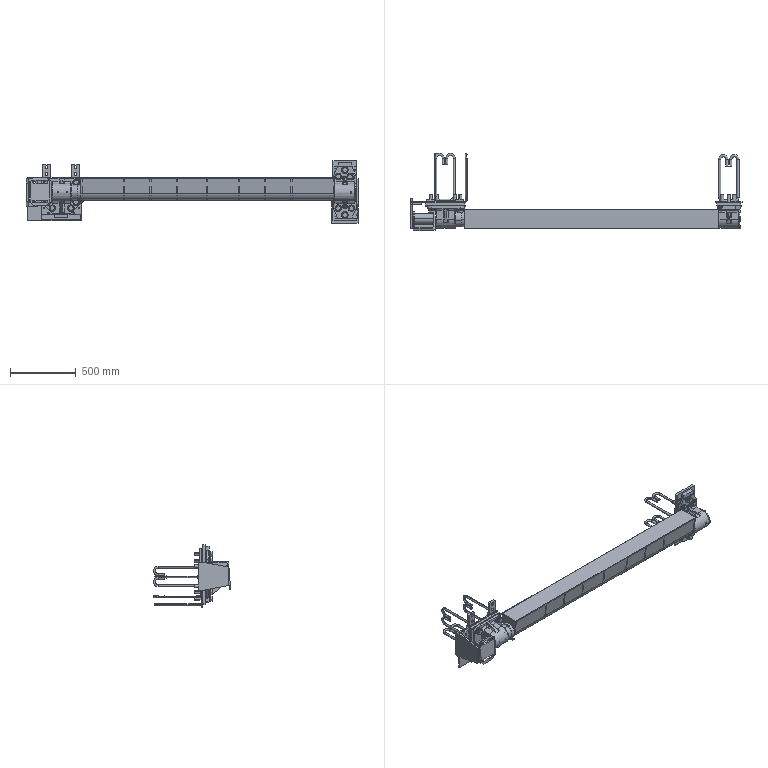Part | SolidWorks | features CompositeCurve 1 | 115 solids | 1909 faces | box 2523 x 586.761 x 475 mm | volume 29684490 mm3 | plane 784 | cylinder 732 | cone 215 | torus 118 | sphere 48 | spline 12 | commonest cylinder face diameters 24 x66 16 x54 10 x48 17.5 x48 12 x44 20 x36